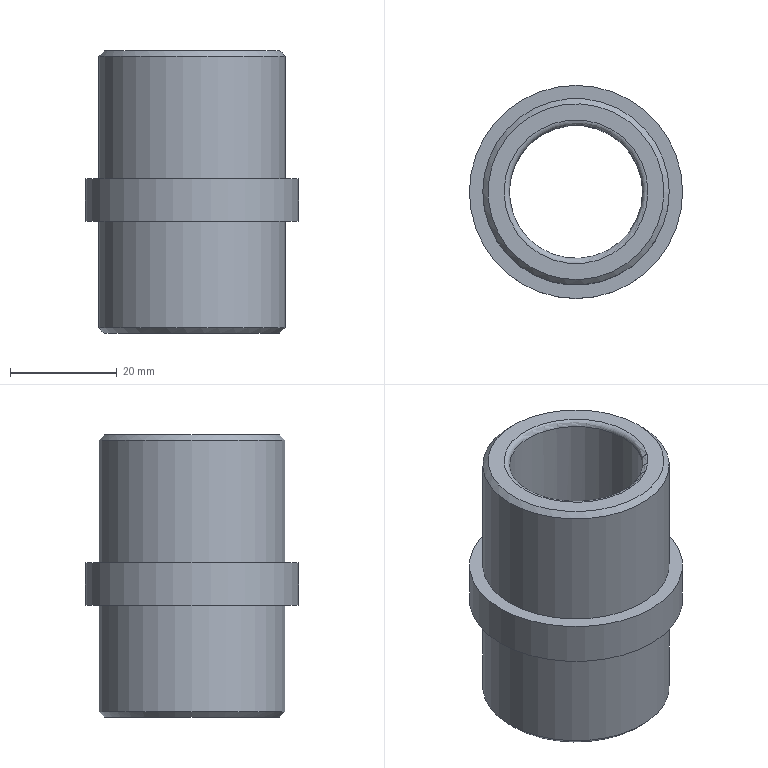Part | STEP file | solid 56 | 1 solid | 12 faces | box 40 x 40 x 53 mm | volume 27190 mm3 | plane 4 | cylinder 4 | cone 2 | torus 2 | commonest cylinder face diameters 35 x2 25 x1 40 x1